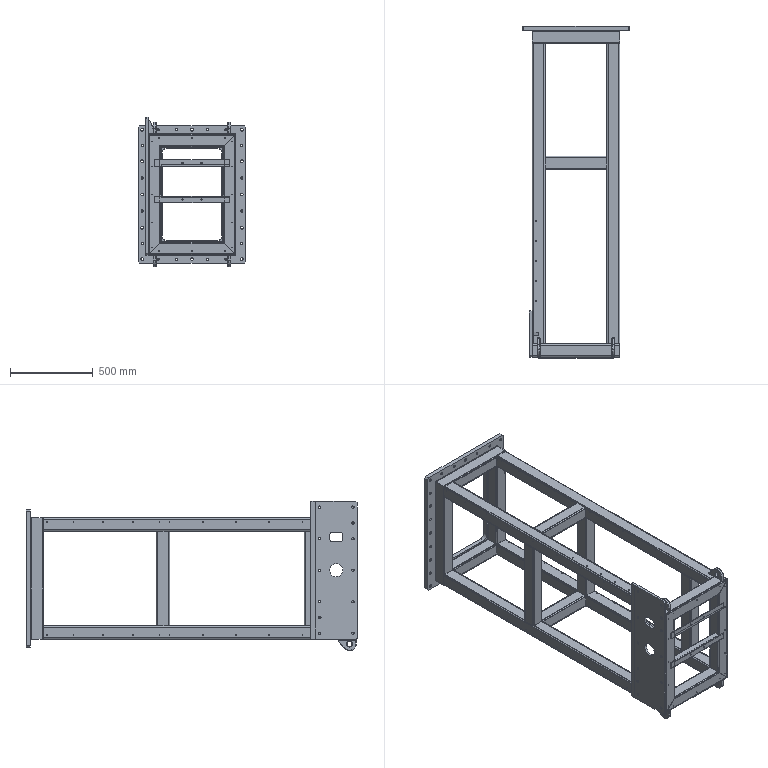Part | SolidWorks | 23 solids | 822 faces | box 650 x 2000 x 900 mm | volume 28576602 mm3 | cylinder 534 | plane 252 | torus 24 | sphere 8 | cone 4 | commonest cylinder face diameters 3.3 x228 16 x72 8 x68 14 x54 6 x28 16.5 x24